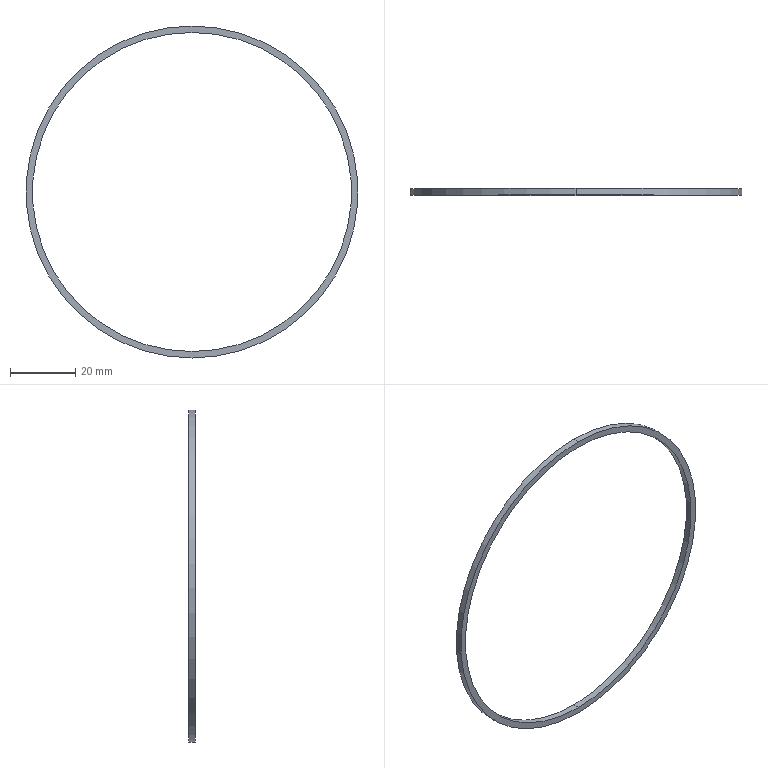Part | NX | features BREP 1 | 1 solid | 6 faces | box 102 x 2 x 102 mm | volume 1257 mm3 | cylinder 4 | plane 2 | commonest cylinder face diameters 98 x2 102 x2
STEP:
#1=CARTESIAN_POINT('',(0.,2.,-49.));
#2=VERTEX_POINT('',#1);
#3=CARTESIAN_POINT('',(0.,2.,49.));
#4=VERTEX_POINT('',#3);
#5=CARTESIAN_POINT('',(0.,2.,0.));
#6=DIRECTION('',(0.,1.,0.));
#7=DIRECTION('',(0.,0.,1.));
#8=AXIS2_PLACEMENT_3D('',#5,#6,#7);
#9=CIRCLE('',#8,49.);
#10=EDGE_CURVE('',#2,#4,#9,.T.);
#11=ORIENTED_EDGE('',*,*,#10,.T.);
#12=CARTESIAN_POINT('',(0.,0.,49.));
#13=VERTEX_POINT('',#12);
#14=CARTESIAN_POINT('',(0.,2.,49.));
#15=DIRECTION('',(0.,-1.,0.));
#16=VECTOR('',#15,1000.);
#17=LINE('',#14,#16);
#18=EDGE_CURVE('',#13,#4,#17,.F.);
#19=ORIENTED_EDGE('',*,*,#18,.F.);
#20=CARTESIAN_POINT('',(0.,0.,-49.));
#21=VERTEX_POINT('',#20);
#22=CARTESIAN_POINT('',(0.,0.,0.));
#23=DIRECTION('',(0.,1.,0.));
#24=DIRECTION('',(0.,0.,1.));
#25=AXIS2_PLACEMENT_3D('',#22,#23,#24);
#26=CIRCLE('',#25,49.);
#27=EDGE_CURVE('',#21,#13,#26,.T.);
#28=ORIENTED_EDGE('',*,*,#27,.F.);
#29=CARTESIAN_POINT('',(0.,2.,-49.));
#30=DIRECTION('',(0.,-1.,0.));
#31=VECTOR('',#30,1000.);
#32=LINE('',#29,#31);
#33=EDGE_CURVE('',#21,#2,#32,.F.);
#34=ORIENTED_EDGE('',*,*,#33,.T.);
#35=EDGE_LOOP('',(#11,#19,#28,#34));
#36=FACE_BOUND('',#35,.T.);
#37=CARTESIAN_POINT('',(0.,2.,0.));
#38=DIRECTION('',(0.,-1.,0.));
#39=DIRECTION('',(0.,0.,1.));
#40=AXIS2_PLACEMENT_3D('',#37,#38,#39);
#41=CYLINDRICAL_SURFACE('',#40,49.);
#42=ADVANCED_FACE('',(#36),#41,.F.);
#43=CARTESIAN_POINT('',(0.,2.,51.));
#44=VERTEX_POINT('',#43);
#45=CARTESIAN_POINT('',(0.,2.,-51.));
#46=VERTEX_POINT('',#45);
#47=CARTESIAN_POINT('',(0.,2.,0.));
#48=DIRECTION('',(0.,1.,0.));
#49=DIRECTION('',(0.,0.,1.));
#50=AXIS2_PLACEMENT_3D('',#47,#48,#49);
#51=CIRCLE('',#50,51.);
#52=EDGE_CURVE('',#44,#46,#51,.T.);
#53=ORIENTED_EDGE('',*,*,#52,.F.);
#54=CARTESIAN_POINT('',(0.,0.,51.));
#55=VERTEX_POINT('',#54);
#56=CARTESIAN_POINT('',(0.,2.,51.));
#57=DIRECTION('',(0.,-1.,0.));
#58=VECTOR('',#57,1000.);
#59=LINE('',#56,#58);
#60=EDGE_CURVE('',#55,#44,#59,.F.);
#61=ORIENTED_EDGE('',*,*,#60,.F.);
#62=CARTESIAN_POINT('',(0.,0.,-51.));
#63=VERTEX_POINT('',#62);
#64=CARTESIAN_POINT('',(0.,0.,0.));
#65=DIRECTION('',(0.,1.,0.));
#66=DIRECTION('',(0.,0.,1.));
#67=AXIS2_PLACEMENT_3D('',#64,#65,#66);
#68=CIRCLE('',#67,51.);
#69=EDGE_CURVE('',#55,#63,#68,.T.);
#70=ORIENTED_EDGE('',*,*,#69,.T.);
#71=CARTESIAN_POINT('',(0.,2.,-51.));
#72=DIRECTION('',(0.,-1.,0.));
#73=VECTOR('',#72,1000.);
#74=LINE('',#71,#73);
#75=EDGE_CURVE('',#63,#46,#74,.F.);
#76=ORIENTED_EDGE('',*,*,#75,.T.);
#77=EDGE_LOOP('',(#53,#61,#70,#76));
#78=FACE_BOUND('',#77,.T.);
#79=CARTESIAN_POINT('',(0.,2.,0.));
#80=DIRECTION('',(0.,-1.,0.));
#81=DIRECTION('',(0.,0.,1.));
#82=AXIS2_PLACEMENT_3D('',#79,#80,#81);
#83=CYLINDRICAL_SURFACE('',#82,51.);
#84=ADVANCED_FACE('',(#78),#83,.T.);
#85=CARTESIAN_POINT('',(0.,2.,0.));
#86=DIRECTION('',(0.,1.,0.));
#87=DIRECTION('',(0.,0.,1.));
#88=AXIS2_PLACEMENT_3D('',#85,#86,#87);
#89=CIRCLE('',#88,51.);
#90=EDGE_CURVE('',#46,#44,#89,.T.);
#91=ORIENTED_EDGE('',*,*,#90,.T.);
#92=ORIENTED_EDGE('',*,*,#52,.T.);
#93=EDGE_LOOP('',(#91,#92));
#94=FACE_BOUND('',#93,.T.);
#95=ORIENTED_EDGE('',*,*,#10,.F.);
#96=CARTESIAN_POINT('',(0.,2.,0.));
#97=DIRECTION('',(0.,1.,0.));
#98=DIRECTION('',(0.,0.,1.));
#99=AXIS2_PLACEMENT_3D('',#96,#97,#98);
#100=CIRCLE('',#99,49.);
#101=EDGE_CURVE('',#4,#2,#100,.T.);
#102=ORIENTED_EDGE('',*,*,#101,.F.);
#103=EDGE_LOOP('',(#95,#102));
#104=FACE_BOUND('',#103,.T.);
#105=CARTESIAN_POINT('',(0.,2.,0.));
#106=DIRECTION('',(0.,1.,0.));
#107=DIRECTION('',(0.,0.,1.));
#108=AXIS2_PLACEMENT_3D('',#105,#106,#107);
#109=PLANE('',#108);
#110=ADVANCED_FACE('',(#94,#104),#109,.T.);
#111=CARTESIAN_POINT('',(0.,0.,0.));
#112=DIRECTION('',(0.,1.,0.));
#113=DIRECTION('',(0.,0.,1.));
#114=AXIS2_PLACEMENT_3D('',#111,#112,#113);
#115=CIRCLE('',#114,51.);
#116=EDGE_CURVE('',#63,#55,#115,.T.);
#117=ORIENTED_EDGE('',*,*,#116,.F.);
#118=ORIENTED_EDGE('',*,*,#69,.F.);
#119=EDGE_LOOP('',(#117,#118));
#120=FACE_BOUND('',#119,.T.);
#121=ORIENTED_EDGE('',*,*,#27,.T.);
#122=CARTESIAN_POINT('',(0.,0.,0.));
#123=DIRECTION('',(0.,1.,0.));
#124=DIRECTION('',(0.,0.,1.));
#125=AXIS2_PLACEMENT_3D('',#122,#123,#124);
#126=CIRCLE('',#125,49.);
#127=EDGE_CURVE('',#13,#21,#126,.T.);
#128=ORIENTED_EDGE('',*,*,#127,.T.);
#129=EDGE_LOOP('',(#121,#128));
#130=FACE_BOUND('',#129,.T.);
#131=CARTESIAN_POINT('',(0.,0.,0.));
#132=DIRECTION('',(0.,1.,0.));
#133=DIRECTION('',(0.,0.,1.));
#134=AXIS2_PLACEMENT_3D('',#131,#132,#133);
#135=PLANE('',#134);
#136=ADVANCED_FACE('',(#120,#130),#135,.F.);
#137=ORIENTED_EDGE('',*,*,#60,.T.);
#138=ORIENTED_EDGE('',*,*,#90,.F.);
#139=ORIENTED_EDGE('',*,*,#75,.F.);
#140=ORIENTED_EDGE('',*,*,#116,.T.);
#141=EDGE_LOOP('',(#137,#138,#139,#140));
#142=FACE_BOUND('',#141,.T.);
#143=CARTESIAN_POINT('',(0.,2.,0.));
#144=DIRECTION('',(0.,-1.,0.));
#145=DIRECTION('',(0.,0.,1.));
#146=AXIS2_PLACEMENT_3D('',#143,#144,#145);
#147=CYLINDRICAL_SURFACE('',#146,51.);
#148=ADVANCED_FACE('',(#142),#147,.T.);
#149=ORIENTED_EDGE('',*,*,#18,.T.);
#150=ORIENTED_EDGE('',*,*,#101,.T.);
#151=ORIENTED_EDGE('',*,*,#33,.F.);
#152=ORIENTED_EDGE('',*,*,#127,.F.);
#153=EDGE_LOOP('',(#149,#150,#151,#152));
#154=FACE_BOUND('',#153,.T.);
#155=CARTESIAN_POINT('',(0.,2.,0.));
#156=DIRECTION('',(0.,-1.,0.));
#157=DIRECTION('',(0.,0.,1.));
#158=AXIS2_PLACEMENT_3D('',#155,#156,#157);
#159=CYLINDRICAL_SURFACE('',#158,49.);
#160=ADVANCED_FACE('',(#154),#159,.F.);
#161=CLOSED_SHELL('',(#42,#84,#110,#136,#148,#160));
#162=MANIFOLD_SOLID_BREP('',#161);
#163=(LENGTH_UNIT()NAMED_UNIT(*)SI_UNIT(.MILLI.,.METRE.));
#164=UNCERTAINTY_MEASURE_WITH_UNIT(LENGTH_MEASURE(0.00001),#163,'','');
#165=(NAMED_UNIT(*)PLANE_ANGLE_UNIT()SI_UNIT($,.RADIAN.));
#166=(NAMED_UNIT(*)SI_UNIT($,.STERADIAN.)SOLID_ANGLE_UNIT());
#167=(GEOMETRIC_REPRESENTATION_CONTEXT(3)GLOBAL_UNCERTAINTY_ASSIGNED_CONTEXT((#164))GLOBAL_UNIT_ASSIGNED_CONTEXT((#163,#165,#166))REPRESENTATION_CONTEXT('',''));
#168=ADVANCED_BREP_SHAPE_REPRESENTATION('',(#162),#167);